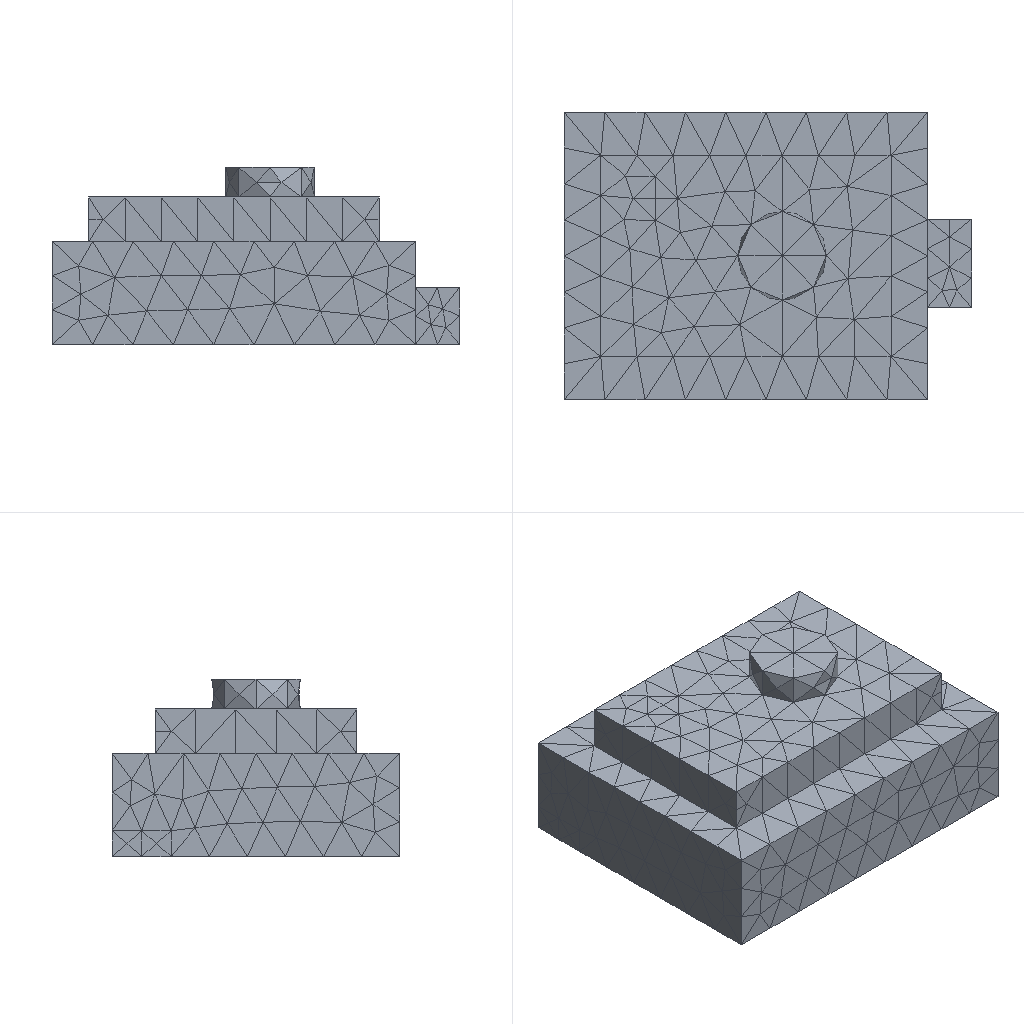Simulation study | ansys mapdl
Set-up summary:
category,name,step,type,value,unit,region
solver,ansys_mapdl
units,mm-N-s-tonne (MPa),,inferred,E=210000 density=
analysis,model,,static
mesh,nodes,,,3889
mesh,elements,,,2276
element_type,SOLID187,,,2276
material,mat 1,,E,210000
material,mat 1,,nu,0.3
load,,model,body load temp,,,all
load,,model,force,"1000 [dir=(0, 0, -1) n=302]",,node list
bc,,model,fixed,"[dofs=UX,UY,UZ n=4606]",,node list
Ansys APDL input file, long lists of numbers shortened:
/COM,ANSYS RELEASE 2026 R1           BUILD 26.1      UP20260202       09:11:07
/PREP7
/NOPR
/TITLE,2
ANTYPE, 0
*IF,_CDRDOFF,EQ,1,THEN     !if solid model was read in
_CDRDOFF=             !reset flag, numoffs already performed
*ELSE              !offset database for the following FE model
NUMOFF,NODE,     3889
NUMOFF,ELEM,     2276
NUMOFF,MAT ,        1
NUMOFF,TYPE,        1
*ENDIF
*SET,_RETURN ,  0.
*SET,_STATUS ,  0.
*SET,_UIQR   ,  302.
*SET,__FLOATPARAMETER__,  3889.
DOF,DELETE
ETBLOCK,        1,        1
(2i9,19a9)
        1      187        0        0        0        0        0        0        0        0        0        0        0        0        0        0        0        0        0        0        0
       -1
NBLOCK,6,SOLID,      3889,      3889
(3i9,6e21.13e3)
        1        0        0-3.3200000000000E+001 3.9000000000000E+001 7.0000000000000E+000
! (3888 more lines like these left out)
N,UNBL,LOC,       -1,
EBLOCK,19,SOLID,      2276,      2276
(19i10)
         1         1         1         1         0         0         0         0        10         0         1      1619      1620      1621      1622      1818      1819      1820      1821
! (4551 more lines like these left out)
        -1
MPTEMP,UNBL, 1, 1,  0.    ,
MPDATA,UNBL, 1,EX  ,       1, 1,  210000.000    ,
MPTEMP,UNBL, 1, 1,  0.    ,
MPDATA,UNBL, 1,NUXY,       1, 1, 0.3    ,
MPTEMP,UNBL, 1, 1,  0.    ,
MPDATA,UNBL, 1,PRXY,       1, 1, 0.3    ,
EXTOPT,ATTR,      0,      0,      0
EXTOPT,ESIZE,  0,  0.
EXTOPT,ACLEAR,      0
TREF,  0.
IRLF,  0
BFUNIF,TEMP,_TINY
ACEL,  0.    ,  0.    ,  0.
OMEGA,  0.    ,  0.    ,  0.
DOMEGA,  0.    ,  0.    ,  0.
CGLOC,  0.    ,  0.    ,  0.
CGOMEGA,  0.    ,  0.    ,  0.
DCGOMG,  0.    ,  0.    ,  0.
KUSE,     0
TIME,  0.
ALPHAD,  0.
BETAD,  0.
DMPRAT,  0.
DMPSTR,  0.
CRPLIM, 0.1    ,   0
CRPLIM,  0.    ,   1
NCNV,     0, 1.000000000E+12,     0,  0.    ,  0.
NEQIT,     0
ERESX,DEFA
DBLOCK,      4606
(i9,a6,2(pg16.9))
        1  UX    0.00000000      0.00000000
! (4605 more lines like these left out)
       -1
FBLOCK,       302
(i9,a6,2(pg16.9))
      487  FZ   -3.31125828      0.00000000
! (301 more lines like these left out)
       -1
/GO
FINISH
Results summary:
result,analysis_type_db,,,static,unstated
result,n_sets,,,1,unstated
result,load_steps[0].set,load_step=1,,1,unstated
result,load_steps[0].substep,load_step=1,,1,unstated
result,load_steps[0].time,load_step=1,,1,unstated
result,load_steps[0].freq,load_step=1,,1,unstated
result,load_steps[0].max_usum,load_step=1,,8.81335e-05,unstated
result,load_steps[0].max_seqv,load_step=1,,1.106,unstated
result,load_steps[0].reaction_sum.FX,load_step=1,,1.62736e-11,unstated
result,load_steps[0].reaction_sum.FY,load_step=1,,-2.27729e-12,unstated
result,load_steps[0].reaction_sum.FZ,load_step=1,,1000,unstated
result,load_steps[0].reaction_sum.MX,load_step=1,,0,unstated
result,load_steps[0].reaction_sum.MY,load_step=1,,0,unstated
result,load_steps[0].reaction_sum.MZ,load_step=1,,0,unstated
result,convergence,,,results present for all listed sets,unstated